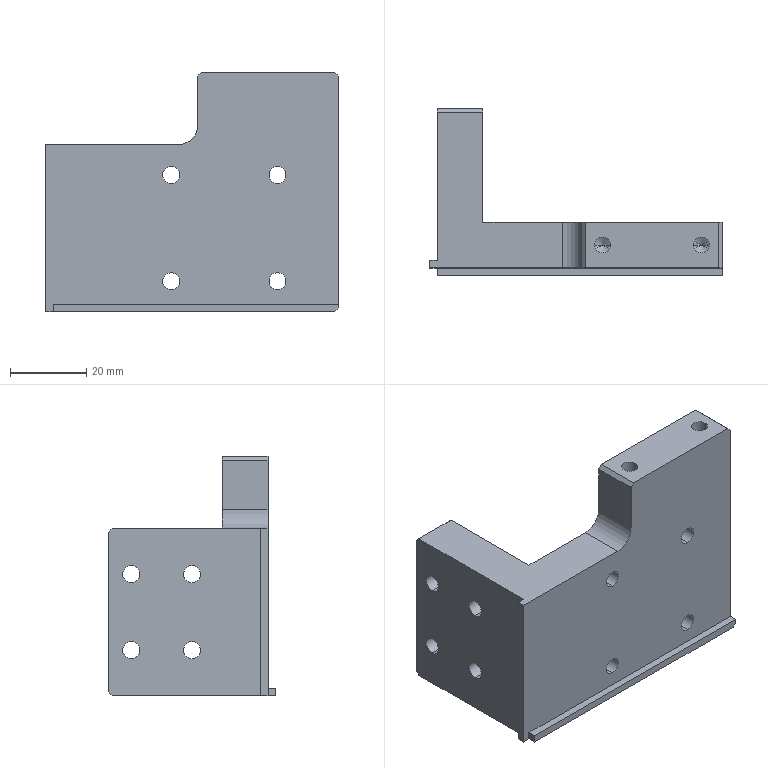Part | SolidWorks | features ICE 6, HoleWzd 4, Chamfer 1, Extrusion 1, Fillet 1 | 1 solid | 69 faces | box 77 x 44 x 63 mm | volume 61294 mm3 | cylinder 37 | plane 28 | cone 4 | commonest cylinder face diameters 4.5 x16 8 x16 4.2 x4 10 x1